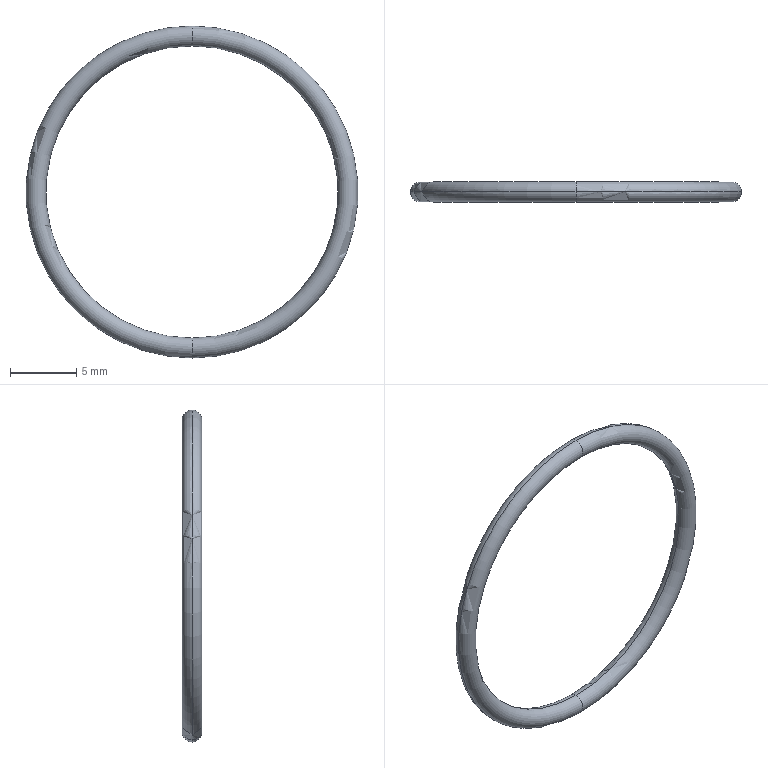Part | SolidWorks | features Revolution 1 | 1 solid | 4 faces | box 25 x 1.5 x 25 mm | volume 130.464 mm3 | torus 4
STEP:
#1=CARTESIAN_POINT('',(0.,0.,12.5));
#2=VERTEX_POINT('',#1);
#3=CARTESIAN_POINT('',(0.,0.,11.));
#4=VERTEX_POINT('',#3);
#5=CARTESIAN_POINT('',(0.,0.,11.75));
#6=DIRECTION('',(1.,0.,0.));
#7=DIRECTION('',(0.,0.,-1.));
#8=AXIS2_PLACEMENT_3D('',#5,#6,#7);
#9=CIRCLE('',#8,0.75);
#10=EDGE_CURVE('',#2,#4,#9,.T.);
#11=ORIENTED_EDGE('',*,*,#10,.F.);
#12=CARTESIAN_POINT('',(0.,0.,-12.5));
#13=VERTEX_POINT('',#12);
#14=CARTESIAN_POINT('',(0.,0.,0.));
#15=DIRECTION('',(0.,-1.,0.));
#16=DIRECTION('',(0.,0.,-1.));
#17=AXIS2_PLACEMENT_3D('',#14,#15,#16);
#18=CIRCLE('',#17,12.5);
#19=EDGE_CURVE('',#2,#13,#18,.T.);
#20=ORIENTED_EDGE('',*,*,#19,.T.);
#21=CARTESIAN_POINT('',(0.,0.,-11.));
#22=VERTEX_POINT('',#21);
#23=CARTESIAN_POINT('',(0.,0.,-11.75));
#24=DIRECTION('',(-1.,0.,0.));
#25=DIRECTION('',(0.,0.,1.));
#26=AXIS2_PLACEMENT_3D('',#23,#24,#25);
#27=CIRCLE('',#26,0.75);
#28=EDGE_CURVE('',#13,#22,#27,.T.);
#29=ORIENTED_EDGE('',*,*,#28,.T.);
#30=CARTESIAN_POINT('',(0.,0.,0.));
#31=DIRECTION('',(0.,-1.,0.));
#32=DIRECTION('',(0.,0.,-1.));
#33=AXIS2_PLACEMENT_3D('',#30,#31,#32);
#34=CIRCLE('',#33,11.);
#35=EDGE_CURVE('',#4,#22,#34,.T.);
#36=ORIENTED_EDGE('',*,*,#35,.F.);
#37=EDGE_LOOP('',(#11,#20,#29,#36));
#38=FACE_OUTER_BOUND('',#37,.T.);
#39=CARTESIAN_POINT('',(0.,0.,0.));
#40=DIRECTION('',(0.,-1.,0.));
#41=DIRECTION('',(0.,0.,-1.));
#42=AXIS2_PLACEMENT_3D('',#39,#40,#41);
#43=TOROIDAL_SURFACE('',#42,11.75,0.75);
#44=ADVANCED_FACE('',(#38),#43,.T.);
#45=ORIENTED_EDGE('',*,*,#28,.F.);
#46=CARTESIAN_POINT('',(0.,0.,0.));
#47=DIRECTION('',(0.,-1.,0.));
#48=DIRECTION('',(0.,0.,-1.));
#49=AXIS2_PLACEMENT_3D('',#46,#47,#48);
#50=CIRCLE('',#49,12.5);
#51=EDGE_CURVE('',#13,#2,#50,.T.);
#52=ORIENTED_EDGE('',*,*,#51,.T.);
#53=ORIENTED_EDGE('',*,*,#10,.T.);
#54=CARTESIAN_POINT('',(0.,0.,0.));
#55=DIRECTION('',(0.,-1.,0.));
#56=DIRECTION('',(0.,0.,-1.));
#57=AXIS2_PLACEMENT_3D('',#54,#55,#56);
#58=CIRCLE('',#57,11.);
#59=EDGE_CURVE('',#22,#4,#58,.T.);
#60=ORIENTED_EDGE('',*,*,#59,.F.);
#61=EDGE_LOOP('',(#45,#52,#53,#60));
#62=FACE_OUTER_BOUND('',#61,.T.);
#63=CARTESIAN_POINT('',(0.,0.,0.));
#64=DIRECTION('',(0.,-1.,0.));
#65=DIRECTION('',(0.,0.,-1.));
#66=AXIS2_PLACEMENT_3D('',#63,#64,#65);
#67=TOROIDAL_SURFACE('',#66,11.75,0.75);
#68=ADVANCED_FACE('',(#62),#67,.T.);
#69=ORIENTED_EDGE('',*,*,#51,.F.);
#70=CARTESIAN_POINT('',(0.,0.,-11.75));
#71=DIRECTION('',(-1.,0.,0.));
#72=DIRECTION('',(0.,0.,1.));
#73=AXIS2_PLACEMENT_3D('',#70,#71,#72);
#74=CIRCLE('',#73,0.75);
#75=EDGE_CURVE('',#22,#13,#74,.T.);
#76=ORIENTED_EDGE('',*,*,#75,.F.);
#77=ORIENTED_EDGE('',*,*,#59,.T.);
#78=CARTESIAN_POINT('',(0.,0.,11.75));
#79=DIRECTION('',(1.,0.,0.));
#80=DIRECTION('',(0.,0.,-1.));
#81=AXIS2_PLACEMENT_3D('',#78,#79,#80);
#82=CIRCLE('',#81,0.75);
#83=EDGE_CURVE('',#4,#2,#82,.T.);
#84=ORIENTED_EDGE('',*,*,#83,.T.);
#85=EDGE_LOOP('',(#69,#76,#77,#84));
#86=FACE_OUTER_BOUND('',#85,.T.);
#87=CARTESIAN_POINT('',(0.,0.,0.));
#88=DIRECTION('',(0.,-1.,0.));
#89=DIRECTION('',(0.,0.,-1.));
#90=AXIS2_PLACEMENT_3D('',#87,#88,#89);
#91=TOROIDAL_SURFACE('',#90,11.75,0.75);
#92=ADVANCED_FACE('',(#86),#91,.T.);
#93=ORIENTED_EDGE('',*,*,#19,.F.);
#94=ORIENTED_EDGE('',*,*,#83,.F.);
#95=ORIENTED_EDGE('',*,*,#35,.T.);
#96=ORIENTED_EDGE('',*,*,#75,.T.);
#97=EDGE_LOOP('',(#93,#94,#95,#96));
#98=FACE_OUTER_BOUND('',#97,.T.);
#99=CARTESIAN_POINT('',(0.,0.,0.));
#100=DIRECTION('',(0.,-1.,0.));
#101=DIRECTION('',(0.,0.,-1.));
#102=AXIS2_PLACEMENT_3D('',#99,#100,#101);
#103=TOROIDAL_SURFACE('',#102,11.75,0.75);
#104=ADVANCED_FACE('',(#98),#103,.T.);
#105=CLOSED_SHELL('',(#44,#68,#92,#104));
#106=MANIFOLD_SOLID_BREP('',#105);
#107=CARTESIAN_POINT('',(0.,0.,0.));
#108=DIRECTION('',(0.,0.,1.));
#109=DIRECTION('',(1.,0.,0.));
#110=AXIS2_PLACEMENT_3D('',#107,#108,#109);
#111=(LENGTH_UNIT()NAMED_UNIT(*)SI_UNIT(.MILLI.,.METRE.));
#112=UNCERTAINTY_MEASURE_WITH_UNIT(LENGTH_MEASURE(0.00001),#111,'','');
#113=(NAMED_UNIT(*)PLANE_ANGLE_UNIT()SI_UNIT($,.RADIAN.));
#114=(NAMED_UNIT(*)SI_UNIT($,.STERADIAN.)SOLID_ANGLE_UNIT());
#115=(GEOMETRIC_REPRESENTATION_CONTEXT(3)GLOBAL_UNCERTAINTY_ASSIGNED_CONTEXT((#112))GLOBAL_UNIT_ASSIGNED_CONTEXT((#111,#113,#114))REPRESENTATION_CONTEXT('',''));
#116=ADVANCED_BREP_SHAPE_REPRESENTATION('',(#106,#110),#115);